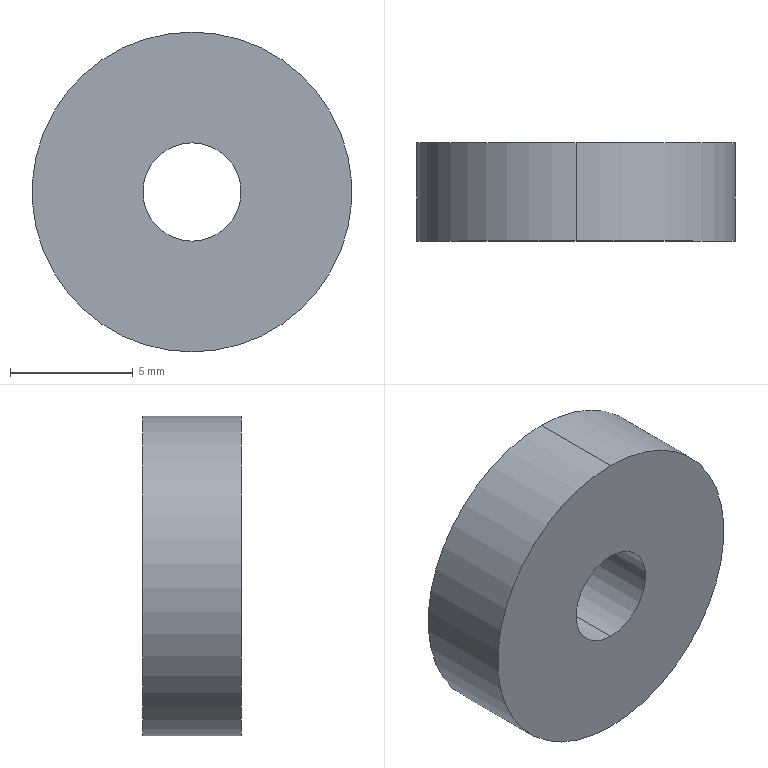Part | SolidWorks | features Revolution 1 | 1 solid | 6 faces | box 13 x 4 x 13 mm | volume 480.664 mm3 | cylinder 4 | plane 2 | commonest cylinder face diameters 4 x2 13 x2
STEP:
#1=CARTESIAN_POINT('',(0.,0.001654,-0.0065));
#2=VERTEX_POINT('',#1);
#3=CARTESIAN_POINT('',(0.,0.001654,0.0065));
#4=VERTEX_POINT('',#3);
#5=CARTESIAN_POINT('',(0.,0.001654,0.));
#6=DIRECTION('',(0.,-1.,0.));
#7=DIRECTION('',(0.,0.,-1.));
#8=AXIS2_PLACEMENT_3D('',#5,#6,#7);
#9=CIRCLE('',#8,0.0065);
#10=EDGE_CURVE('',#2,#4,#9,.T.);
#11=ORIENTED_EDGE('',*,*,#10,.T.);
#12=CARTESIAN_POINT('',(0.,-0.002346,0.0065));
#13=VERTEX_POINT('',#12);
#14=CARTESIAN_POINT('',(0.,0.,0.0065));
#15=DIRECTION('',(0.,-1.,0.));
#16=VECTOR('',#15,1.);
#17=LINE('',#14,#16);
#18=EDGE_CURVE('',#4,#13,#17,.T.);
#19=ORIENTED_EDGE('',*,*,#18,.T.);
#20=CARTESIAN_POINT('',(0.,-0.002346,-0.0065));
#21=VERTEX_POINT('',#20);
#22=CARTESIAN_POINT('',(0.,-0.002346,0.));
#23=DIRECTION('',(0.,-1.,0.));
#24=DIRECTION('',(0.,0.,-1.));
#25=AXIS2_PLACEMENT_3D('',#22,#23,#24);
#26=CIRCLE('',#25,0.0065);
#27=EDGE_CURVE('',#21,#13,#26,.T.);
#28=ORIENTED_EDGE('',*,*,#27,.F.);
#29=CARTESIAN_POINT('',(0.,0.,-0.0065));
#30=DIRECTION('',(0.,-1.,0.));
#31=VECTOR('',#30,1.);
#32=LINE('',#29,#31);
#33=EDGE_CURVE('',#2,#21,#32,.T.);
#34=ORIENTED_EDGE('',*,*,#33,.F.);
#35=EDGE_LOOP('',(#11,#19,#28,#34));
#36=FACE_OUTER_BOUND('',#35,.T.);
#37=CARTESIAN_POINT('',(0.,0.,0.));
#38=DIRECTION('',(0.,-1.,0.));
#39=DIRECTION('',(0.,0.,-1.));
#40=AXIS2_PLACEMENT_3D('',#37,#38,#39);
#41=CYLINDRICAL_SURFACE('',#40,0.0065);
#42=ADVANCED_FACE('',(#36),#41,.T.);
#43=CARTESIAN_POINT('',(0.,0.001654,0.002));
#44=VERTEX_POINT('',#43);
#45=CARTESIAN_POINT('',(0.,0.001654,-0.002));
#46=VERTEX_POINT('',#45);
#47=CARTESIAN_POINT('',(0.,0.001654,0.));
#48=DIRECTION('',(0.,-1.,0.));
#49=DIRECTION('',(0.,0.,-1.));
#50=AXIS2_PLACEMENT_3D('',#47,#48,#49);
#51=CIRCLE('',#50,0.002);
#52=EDGE_CURVE('',#44,#46,#51,.T.);
#53=ORIENTED_EDGE('',*,*,#52,.F.);
#54=CARTESIAN_POINT('',(0.,-0.002346,0.002));
#55=VERTEX_POINT('',#54);
#56=CARTESIAN_POINT('',(0.,0.,0.002));
#57=DIRECTION('',(0.,-1.,0.));
#58=VECTOR('',#57,1.);
#59=LINE('',#56,#58);
#60=EDGE_CURVE('',#44,#55,#59,.T.);
#61=ORIENTED_EDGE('',*,*,#60,.T.);
#62=CARTESIAN_POINT('',(0.,-0.002346,-0.002));
#63=VERTEX_POINT('',#62);
#64=CARTESIAN_POINT('',(0.,-0.002346,0.));
#65=DIRECTION('',(0.,-1.,0.));
#66=DIRECTION('',(0.,0.,-1.));
#67=AXIS2_PLACEMENT_3D('',#64,#65,#66);
#68=CIRCLE('',#67,0.002);
#69=EDGE_CURVE('',#55,#63,#68,.T.);
#70=ORIENTED_EDGE('',*,*,#69,.T.);
#71=CARTESIAN_POINT('',(0.,0.,-0.002));
#72=DIRECTION('',(0.,-1.,0.));
#73=VECTOR('',#72,1.);
#74=LINE('',#71,#73);
#75=EDGE_CURVE('',#46,#63,#74,.T.);
#76=ORIENTED_EDGE('',*,*,#75,.F.);
#77=EDGE_LOOP('',(#53,#61,#70,#76));
#78=FACE_OUTER_BOUND('',#77,.T.);
#79=CARTESIAN_POINT('',(0.,0.,0.));
#80=DIRECTION('',(0.,-1.,0.));
#81=DIRECTION('',(0.,0.,-1.));
#82=AXIS2_PLACEMENT_3D('',#79,#80,#81);
#83=CYLINDRICAL_SURFACE('',#82,0.002);
#84=ADVANCED_FACE('',(#78),#83,.F.);
#85=ORIENTED_EDGE('',*,*,#60,.F.);
#86=CARTESIAN_POINT('',(0.,0.001654,0.));
#87=DIRECTION('',(0.,-1.,0.));
#88=DIRECTION('',(0.,0.,-1.));
#89=AXIS2_PLACEMENT_3D('',#86,#87,#88);
#90=CIRCLE('',#89,0.002);
#91=EDGE_CURVE('',#46,#44,#90,.T.);
#92=ORIENTED_EDGE('',*,*,#91,.F.);
#93=ORIENTED_EDGE('',*,*,#75,.T.);
#94=CARTESIAN_POINT('',(0.,-0.002346,0.));
#95=DIRECTION('',(0.,-1.,0.));
#96=DIRECTION('',(0.,0.,-1.));
#97=AXIS2_PLACEMENT_3D('',#94,#95,#96);
#98=CIRCLE('',#97,0.002);
#99=EDGE_CURVE('',#63,#55,#98,.T.);
#100=ORIENTED_EDGE('',*,*,#99,.T.);
#101=EDGE_LOOP('',(#85,#92,#93,#100));
#102=FACE_OUTER_BOUND('',#101,.T.);
#103=CARTESIAN_POINT('',(0.,0.,0.));
#104=DIRECTION('',(0.,-1.,0.));
#105=DIRECTION('',(0.,0.,-1.));
#106=AXIS2_PLACEMENT_3D('',#103,#104,#105);
#107=CYLINDRICAL_SURFACE('',#106,0.002);
#108=ADVANCED_FACE('',(#102),#107,.F.);
#109=ORIENTED_EDGE('',*,*,#27,.T.);
#110=CARTESIAN_POINT('',(0.,-0.002346,0.));
#111=DIRECTION('',(0.,-1.,0.));
#112=DIRECTION('',(0.,0.,-1.));
#113=AXIS2_PLACEMENT_3D('',#110,#111,#112);
#114=CIRCLE('',#113,0.0065);
#115=EDGE_CURVE('',#13,#21,#114,.T.);
#116=ORIENTED_EDGE('',*,*,#115,.T.);
#117=EDGE_LOOP('',(#109,#116));
#118=FACE_OUTER_BOUND('',#117,.T.);
#119=ORIENTED_EDGE('',*,*,#99,.F.);
#120=ORIENTED_EDGE('',*,*,#69,.F.);
#121=EDGE_LOOP('',(#119,#120));
#122=FACE_BOUND('',#121,.T.);
#123=CARTESIAN_POINT('',(0.002,-0.002346,0.));
#124=DIRECTION('',(0.,-1.,0.));
#125=DIRECTION('',(0.,0.,-1.));
#126=AXIS2_PLACEMENT_3D('',#123,#124,#125);
#127=PLANE('',#126);
#128=ADVANCED_FACE('',(#118,#122),#127,.T.);
#129=ORIENTED_EDGE('',*,*,#18,.F.);
#130=CARTESIAN_POINT('',(0.,0.001654,0.));
#131=DIRECTION('',(0.,-1.,0.));
#132=DIRECTION('',(0.,0.,-1.));
#133=AXIS2_PLACEMENT_3D('',#130,#131,#132);
#134=CIRCLE('',#133,0.0065);
#135=EDGE_CURVE('',#4,#2,#134,.T.);
#136=ORIENTED_EDGE('',*,*,#135,.T.);
#137=ORIENTED_EDGE('',*,*,#33,.T.);
#138=ORIENTED_EDGE('',*,*,#115,.F.);
#139=EDGE_LOOP('',(#129,#136,#137,#138));
#140=FACE_OUTER_BOUND('',#139,.T.);
#141=CARTESIAN_POINT('',(0.,0.,0.));
#142=DIRECTION('',(0.,-1.,0.));
#143=DIRECTION('',(0.,0.,-1.));
#144=AXIS2_PLACEMENT_3D('',#141,#142,#143);
#145=CYLINDRICAL_SURFACE('',#144,0.0065);
#146=ADVANCED_FACE('',(#140),#145,.T.);
#147=ORIENTED_EDGE('',*,*,#91,.T.);
#148=ORIENTED_EDGE('',*,*,#52,.T.);
#149=EDGE_LOOP('',(#147,#148));
#150=FACE_BOUND('',#149,.T.);
#151=ORIENTED_EDGE('',*,*,#10,.F.);
#152=ORIENTED_EDGE('',*,*,#135,.F.);
#153=EDGE_LOOP('',(#151,#152));
#154=FACE_OUTER_BOUND('',#153,.T.);
#155=CARTESIAN_POINT('',(0.002,0.001654,0.));
#156=DIRECTION('',(0.,1.,0.));
#157=DIRECTION('',(0.,0.,1.));
#158=AXIS2_PLACEMENT_3D('',#155,#156,#157);
#159=PLANE('',#158);
#160=ADVANCED_FACE('',(#150,#154),#159,.T.);
#161=CLOSED_SHELL('',(#42,#84,#108,#128,#146,#160));
#162=MANIFOLD_SOLID_BREP('',#161);
#163=CARTESIAN_POINT('',(0.,0.,0.));
#164=DIRECTION('',(0.,0.,1.));
#165=DIRECTION('',(1.,0.,0.));
#166=AXIS2_PLACEMENT_3D('',#163,#164,#165);
#167=(LENGTH_UNIT()NAMED_UNIT(*)SI_UNIT($,.METRE.));
#168=UNCERTAINTY_MEASURE_WITH_UNIT(LENGTH_MEASURE(0.00001),#167,'','');
#169=(NAMED_UNIT(*)PLANE_ANGLE_UNIT()SI_UNIT($,.RADIAN.));
#170=(NAMED_UNIT(*)SI_UNIT($,.STERADIAN.)SOLID_ANGLE_UNIT());
#171=(GEOMETRIC_REPRESENTATION_CONTEXT(3)GLOBAL_UNCERTAINTY_ASSIGNED_CONTEXT((#168))GLOBAL_UNIT_ASSIGNED_CONTEXT((#167,#169,#170))REPRESENTATION_CONTEXT('',''));
#172=ADVANCED_BREP_SHAPE_REPRESENTATION('',(#162,#166),#171);